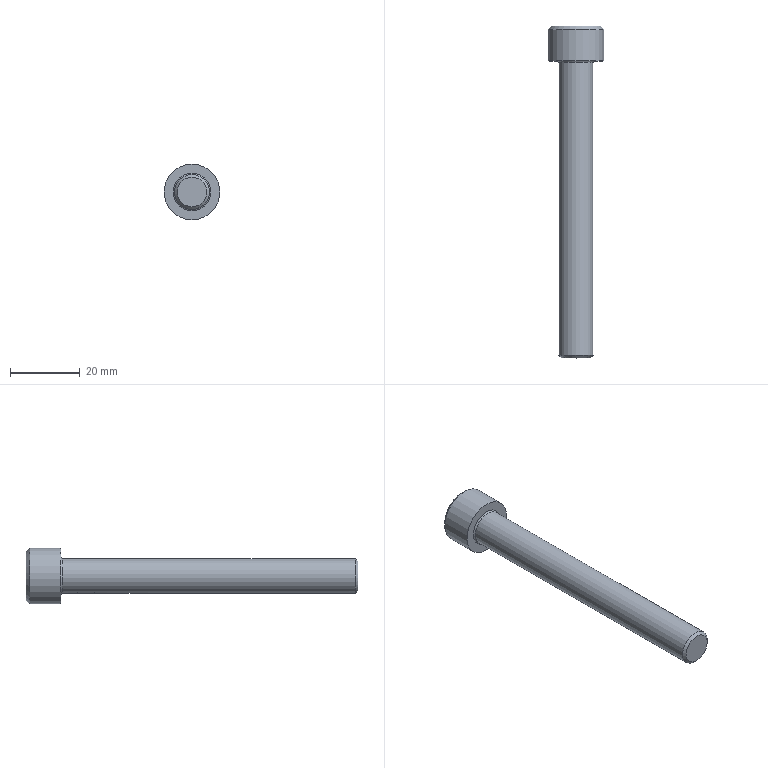Part | STEP file | solid 52 | 1 solid | 112 faces | box 16 x 95 x 16 mm | volume 8373 mm3 | plane 58 | other 37 | cylinder 8 | sphere 6 | cone 2 | torus 1 | commonest cylinder face diameters 10 x7 16 x1